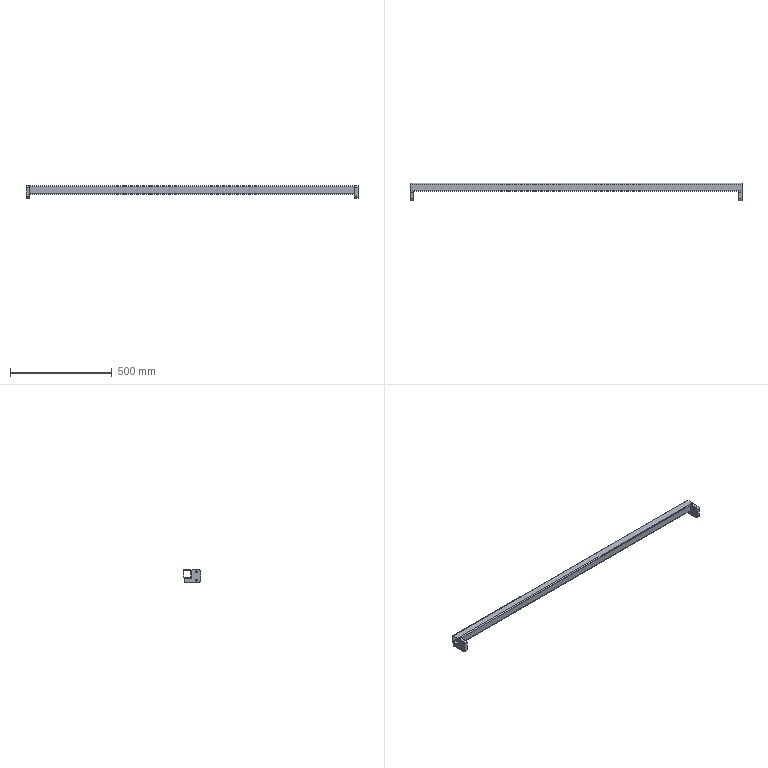Part | SolidWorks | features BaseBody 3 | 3 solids | 52 faces | box 1632 x 85 x 60 mm | volume 797104 mm3 | plane 26 | cylinder 26 | commonest cylinder face diameters 10 x8 10.2 x8 4 x4 20 x4 6 x2